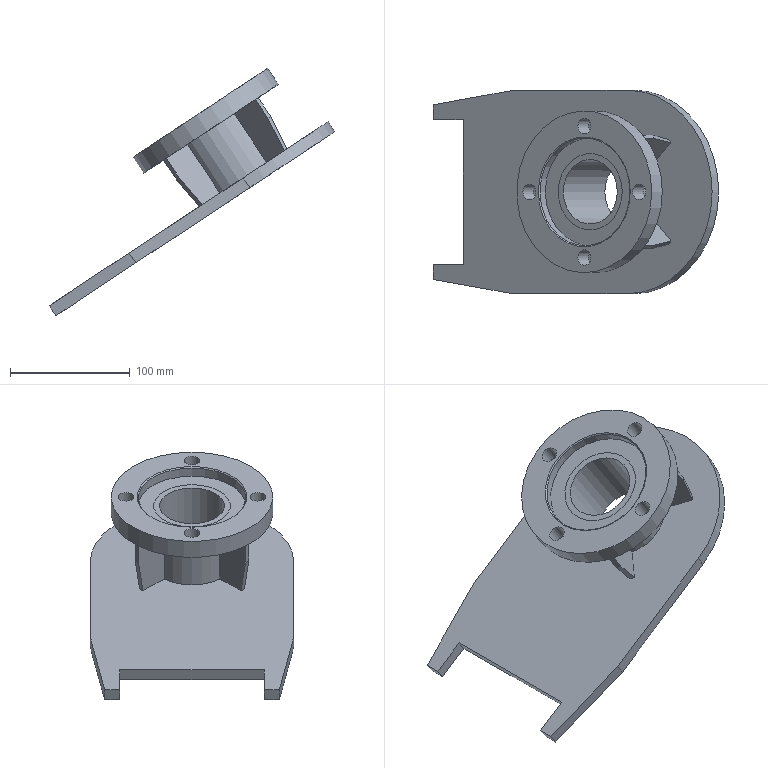Part | STEP file | HL4GZ-1.862.036MP (roller mounting base) | 7 solids | 61 faces | box 238.392 x 170 x 206.608 mm | volume 617379 mm3 | plane 46 | cylinder 13 | cone 2 | commonest cylinder face diameters 13 x4 64 x4 54 x1 70 x1 90 x1 135 x1